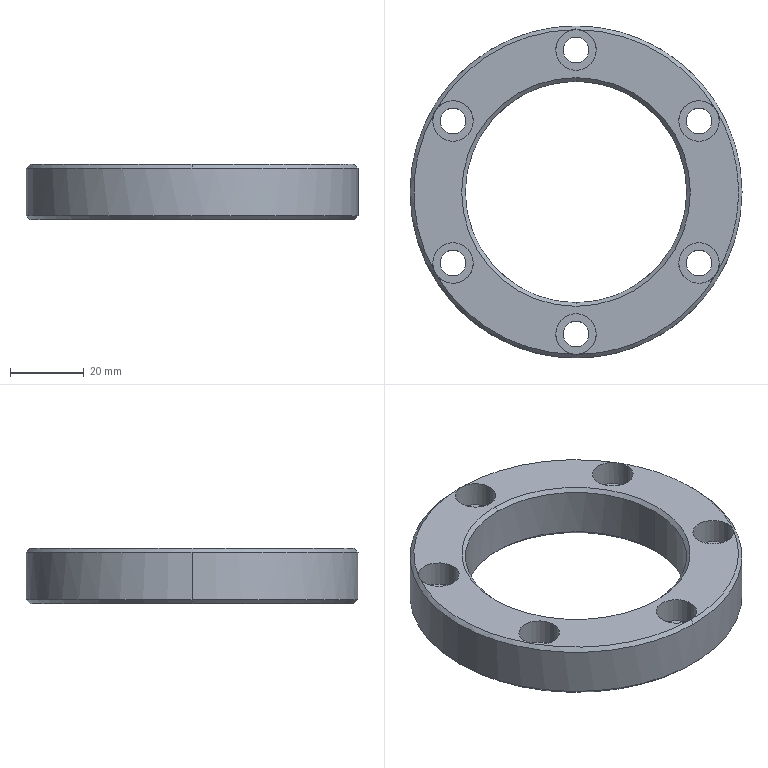Part | STEP file | End Cover | 1 solid | 44 faces | box 90 x 90 x 15 mm | volume 46704 mm3 | cylinder 28 | cone 8 | plane 8 | commonest cylinder face diameters 7 x12 11 x12 60 x2 90 x2
STEP:
#1=CARTESIAN_POINT('',(-29.842,19.25,8.));
#2=VERTEX_POINT('',#1);
#3=CARTESIAN_POINT('',(-36.842,19.25,8.));
#4=VERTEX_POINT('',#3);
#5=CARTESIAN_POINT('',(-33.342,19.25,8.));
#6=DIRECTION('',(0.,0.,-1.));
#7=DIRECTION('',(-1.,0.,0.));
#8=AXIS2_PLACEMENT_3D('',#5,#6,#7);
#9=CIRCLE('',#8,3.5);
#10=EDGE_CURVE('',#2,#4,#9,.T.);
#11=ORIENTED_EDGE('',*,*,#10,.F.);
#12=CARTESIAN_POINT('',(-29.842,19.25,0.));
#13=VERTEX_POINT('',#12);
#14=CARTESIAN_POINT('',(-29.842,19.25,15.));
#15=DIRECTION('',(0.,0.,-1.));
#16=VECTOR('',#15,1000.);
#17=LINE('',#14,#16);
#18=EDGE_CURVE('',#2,#13,#17,.T.);
#19=ORIENTED_EDGE('',*,*,#18,.T.);
#20=CARTESIAN_POINT('',(-36.842,19.25,0.));
#21=VERTEX_POINT('',#20);
#22=CARTESIAN_POINT('',(-33.342,19.25,0.));
#23=DIRECTION('',(0.,0.,-1.));
#24=DIRECTION('',(-1.,0.,0.));
#25=AXIS2_PLACEMENT_3D('',#22,#23,#24);
#26=CIRCLE('',#25,3.5);
#27=EDGE_CURVE('',#13,#21,#26,.T.);
#28=ORIENTED_EDGE('',*,*,#27,.T.);
#29=CARTESIAN_POINT('',(-36.842,19.25,15.));
#30=DIRECTION('',(0.,0.,-1.));
#31=VECTOR('',#30,1000.);
#32=LINE('',#29,#31);
#33=EDGE_CURVE('',#4,#21,#32,.T.);
#34=ORIENTED_EDGE('',*,*,#33,.F.);
#35=EDGE_LOOP('',(#11,#19,#28,#34));
#36=FACE_OUTER_BOUND('',#35,.T.);
#37=CARTESIAN_POINT('',(-33.342,19.25,15.));
#38=DIRECTION('',(0.,0.,-1.));
#39=DIRECTION('',(-1.,0.,0.));
#40=AXIS2_PLACEMENT_3D('',#37,#38,#39);
#41=CYLINDRICAL_SURFACE('',#40,3.5);
#42=ADVANCED_FACE('',(#36),#41,.F.);
#43=CARTESIAN_POINT('',(3.5,-38.5,8.));
#44=VERTEX_POINT('',#43);
#45=CARTESIAN_POINT('',(-3.5,-38.5,8.));
#46=VERTEX_POINT('',#45);
#47=CARTESIAN_POINT('',(0.,-38.5,8.));
#48=DIRECTION('',(0.,0.,-1.));
#49=DIRECTION('',(-1.,0.,0.));
#50=AXIS2_PLACEMENT_3D('',#47,#48,#49);
#51=CIRCLE('',#50,3.5);
#52=EDGE_CURVE('',#44,#46,#51,.T.);
#53=ORIENTED_EDGE('',*,*,#52,.F.);
#54=CARTESIAN_POINT('',(3.5,-38.5,0.));
#55=VERTEX_POINT('',#54);
#56=CARTESIAN_POINT('',(3.5,-38.5,15.));
#57=DIRECTION('',(0.,0.,-1.));
#58=VECTOR('',#57,1000.);
#59=LINE('',#56,#58);
#60=EDGE_CURVE('',#44,#55,#59,.T.);
#61=ORIENTED_EDGE('',*,*,#60,.T.);
#62=CARTESIAN_POINT('',(-3.5,-38.5,0.));
#63=VERTEX_POINT('',#62);
#64=CARTESIAN_POINT('',(0.,-38.5,0.));
#65=DIRECTION('',(0.,0.,-1.));
#66=DIRECTION('',(-1.,0.,0.));
#67=AXIS2_PLACEMENT_3D('',#64,#65,#66);
#68=CIRCLE('',#67,3.5);
#69=EDGE_CURVE('',#55,#63,#68,.T.);
#70=ORIENTED_EDGE('',*,*,#69,.T.);
#71=CARTESIAN_POINT('',(-3.5,-38.5,15.));
#72=DIRECTION('',(0.,0.,-1.));
#73=VECTOR('',#72,1000.);
#74=LINE('',#71,#73);
#75=EDGE_CURVE('',#46,#63,#74,.T.);
#76=ORIENTED_EDGE('',*,*,#75,.F.);
#77=EDGE_LOOP('',(#53,#61,#70,#76));
#78=FACE_OUTER_BOUND('',#77,.T.);
#79=CARTESIAN_POINT('',(0.,-38.5,15.));
#80=DIRECTION('',(0.,0.,-1.));
#81=DIRECTION('',(-1.,0.,0.));
#82=AXIS2_PLACEMENT_3D('',#79,#80,#81);
#83=CYLINDRICAL_SURFACE('',#82,3.5);
#84=ADVANCED_FACE('',(#78),#83,.F.);
#85=CARTESIAN_POINT('',(36.842,19.25,8.));
#86=VERTEX_POINT('',#85);
#87=CARTESIAN_POINT('',(29.842,19.25,8.));
#88=VERTEX_POINT('',#87);
#89=CARTESIAN_POINT('',(33.342,19.25,8.));
#90=DIRECTION('',(0.,0.,-1.));
#91=DIRECTION('',(-1.,0.,0.));
#92=AXIS2_PLACEMENT_3D('',#89,#90,#91);
#93=CIRCLE('',#92,3.5);
#94=EDGE_CURVE('',#86,#88,#93,.T.);
#95=ORIENTED_EDGE('',*,*,#94,.F.);
#96=CARTESIAN_POINT('',(36.842,19.25,0.));
#97=VERTEX_POINT('',#96);
#98=CARTESIAN_POINT('',(36.842,19.25,15.));
#99=DIRECTION('',(0.,0.,-1.));
#100=VECTOR('',#99,1000.);
#101=LINE('',#98,#100);
#102=EDGE_CURVE('',#86,#97,#101,.T.);
#103=ORIENTED_EDGE('',*,*,#102,.T.);
#104=CARTESIAN_POINT('',(29.842,19.25,0.));
#105=VERTEX_POINT('',#104);
#106=CARTESIAN_POINT('',(33.342,19.25,0.));
#107=DIRECTION('',(0.,0.,-1.));
#108=DIRECTION('',(-1.,0.,0.));
#109=AXIS2_PLACEMENT_3D('',#106,#107,#108);
#110=CIRCLE('',#109,3.5);
#111=EDGE_CURVE('',#97,#105,#110,.T.);
#112=ORIENTED_EDGE('',*,*,#111,.T.);
#113=CARTESIAN_POINT('',(29.842,19.25,15.));
#114=DIRECTION('',(0.,0.,-1.));
#115=VECTOR('',#114,1000.);
#116=LINE('',#113,#115);
#117=EDGE_CURVE('',#88,#105,#116,.T.);
#118=ORIENTED_EDGE('',*,*,#117,.F.);
#119=EDGE_LOOP('',(#95,#103,#112,#118));
#120=FACE_OUTER_BOUND('',#119,.T.);
#121=CARTESIAN_POINT('',(33.342,19.25,15.));
#122=DIRECTION('',(0.,0.,-1.));
#123=DIRECTION('',(-1.,0.,0.));
#124=AXIS2_PLACEMENT_3D('',#121,#122,#123);
#125=CYLINDRICAL_SURFACE('',#124,3.5);
#126=ADVANCED_FACE('',(#120),#125,.F.);
#127=CARTESIAN_POINT('',(3.5,38.5,8.));
#128=VERTEX_POINT('',#127);
#129=CARTESIAN_POINT('',(-3.5,38.5,8.));
#130=VERTEX_POINT('',#129);
#131=CARTESIAN_POINT('',(0.,38.5,8.));
#132=DIRECTION('',(0.,0.,-1.));
#133=DIRECTION('',(-1.,0.,0.));
#134=AXIS2_PLACEMENT_3D('',#131,#132,#133);
#135=CIRCLE('',#134,3.5);
#136=EDGE_CURVE('',#128,#130,#135,.T.);
#137=ORIENTED_EDGE('',*,*,#136,.F.);
#138=CARTESIAN_POINT('',(3.5,38.5,0.));
#139=VERTEX_POINT('',#138);
#140=CARTESIAN_POINT('',(3.5,38.5,15.));
#141=DIRECTION('',(0.,0.,-1.));
#142=VECTOR('',#141,1000.);
#143=LINE('',#140,#142);
#144=EDGE_CURVE('',#128,#139,#143,.T.);
#145=ORIENTED_EDGE('',*,*,#144,.T.);
#146=CARTESIAN_POINT('',(-3.5,38.5,0.));
#147=VERTEX_POINT('',#146);
#148=CARTESIAN_POINT('',(0.,38.5,0.));
#149=DIRECTION('',(0.,0.,-1.));
#150=DIRECTION('',(-1.,0.,0.));
#151=AXIS2_PLACEMENT_3D('',#148,#149,#150);
#152=CIRCLE('',#151,3.5);
#153=EDGE_CURVE('',#139,#147,#152,.T.);
#154=ORIENTED_EDGE('',*,*,#153,.T.);
#155=CARTESIAN_POINT('',(-3.5,38.5,15.));
#156=DIRECTION('',(0.,0.,-1.));
#157=VECTOR('',#156,1000.);
#158=LINE('',#155,#157);
#159=EDGE_CURVE('',#130,#147,#158,.T.);
#160=ORIENTED_EDGE('',*,*,#159,.F.);
#161=EDGE_LOOP('',(#137,#145,#154,#160));
#162=FACE_OUTER_BOUND('',#161,.T.);
#163=CARTESIAN_POINT('',(0.,38.5,15.));
#164=DIRECTION('',(0.,0.,-1.));
#165=DIRECTION('',(-1.,0.,0.));
#166=AXIS2_PLACEMENT_3D('',#163,#164,#165);
#167=CYLINDRICAL_SURFACE('',#166,3.5);
#168=ADVANCED_FACE('',(#162),#167,.F.);
#169=CARTESIAN_POINT('',(36.842,-19.25,8.));
#170=VERTEX_POINT('',#169);
#171=CARTESIAN_POINT('',(29.842,-19.25,8.));
#172=VERTEX_POINT('',#171);
#173=CARTESIAN_POINT('',(33.342,-19.25,8.));
#174=DIRECTION('',(0.,0.,-1.));
#175=DIRECTION('',(-1.,0.,0.));
#176=AXIS2_PLACEMENT_3D('',#173,#174,#175);
#177=CIRCLE('',#176,3.5);
#178=EDGE_CURVE('',#170,#172,#177,.T.);
#179=ORIENTED_EDGE('',*,*,#178,.F.);
#180=CARTESIAN_POINT('',(36.842,-19.25,0.));
#181=VERTEX_POINT('',#180);
#182=CARTESIAN_POINT('',(36.842,-19.25,15.));
#183=DIRECTION('',(0.,0.,-1.));
#184=VECTOR('',#183,1000.);
#185=LINE('',#182,#184);
#186=EDGE_CURVE('',#170,#181,#185,.T.);
#187=ORIENTED_EDGE('',*,*,#186,.T.);
#188=CARTESIAN_POINT('',(29.842,-19.25,0.));
#189=VERTEX_POINT('',#188);
#190=CARTESIAN_POINT('',(33.342,-19.25,0.));
#191=DIRECTION('',(0.,0.,-1.));
#192=DIRECTION('',(-1.,0.,0.));
#193=AXIS2_PLACEMENT_3D('',#190,#191,#192);
#194=CIRCLE('',#193,3.5);
#195=EDGE_CURVE('',#181,#189,#194,.T.);
#196=ORIENTED_EDGE('',*,*,#195,.T.);
#197=CARTESIAN_POINT('',(29.842,-19.25,15.));
#198=DIRECTION('',(0.,0.,-1.));
#199=VECTOR('',#198,1000.);
#200=LINE('',#197,#199);
#201=EDGE_CURVE('',#172,#189,#200,.T.);
#202=ORIENTED_EDGE('',*,*,#201,.F.);
#203=EDGE_LOOP('',(#179,#187,#196,#202));
#204=FACE_OUTER_BOUND('',#203,.T.);
#205=CARTESIAN_POINT('',(33.342,-19.25,15.));
#206=DIRECTION('',(0.,0.,-1.));
#207=DIRECTION('',(-1.,0.,0.));
#208=AXIS2_PLACEMENT_3D('',#205,#206,#207);
#209=CYLINDRICAL_SURFACE('',#208,3.5);
#210=ADVANCED_FACE('',(#204),#209,.F.);
#211=CARTESIAN_POINT('',(-29.842,-19.25,8.));
#212=VERTEX_POINT('',#211);
#213=CARTESIAN_POINT('',(-36.842,-19.25,8.));
#214=VERTEX_POINT('',#213);
#215=CARTESIAN_POINT('',(-33.342,-19.25,8.));
#216=DIRECTION('',(0.,0.,-1.));
#217=DIRECTION('',(-1.,0.,0.));
#218=AXIS2_PLACEMENT_3D('',#215,#216,#217);
#219=CIRCLE('',#218,3.5);
#220=EDGE_CURVE('',#212,#214,#219,.T.);
#221=ORIENTED_EDGE('',*,*,#220,.F.);
#222=CARTESIAN_POINT('',(-29.842,-19.25,0.));
#223=VERTEX_POINT('',#222);
#224=CARTESIAN_POINT('',(-29.842,-19.25,15.));
#225=DIRECTION('',(0.,0.,-1.));
#226=VECTOR('',#225,1000.);
#227=LINE('',#224,#226);
#228=EDGE_CURVE('',#212,#223,#227,.T.);
#229=ORIENTED_EDGE('',*,*,#228,.T.);
#230=CARTESIAN_POINT('',(-36.842,-19.25,0.));
#231=VERTEX_POINT('',#230);
#232=CARTESIAN_POINT('',(-33.342,-19.25,0.));
#233=DIRECTION('',(0.,0.,-1.));
#234=DIRECTION('',(-1.,0.,0.));
#235=AXIS2_PLACEMENT_3D('',#232,#233,#234);
#236=CIRCLE('',#235,3.5);
#237=EDGE_CURVE('',#223,#231,#236,.T.);
#238=ORIENTED_EDGE('',*,*,#237,.T.);
#239=CARTESIAN_POINT('',(-36.842,-19.25,15.));
#240=DIRECTION('',(0.,0.,-1.));
#241=VECTOR('',#240,1000.);
#242=LINE('',#239,#241);
#243=EDGE_CURVE('',#214,#231,#242,.T.);
#244=ORIENTED_EDGE('',*,*,#243,.F.);
#245=EDGE_LOOP('',(#221,#229,#238,#244));
#246=FACE_OUTER_BOUND('',#245,.T.);
#247=CARTESIAN_POINT('',(-33.342,-19.25,15.));
#248=DIRECTION('',(0.,0.,-1.));
#249=DIRECTION('',(-1.,0.,0.));
#250=AXIS2_PLACEMENT_3D('',#247,#248,#249);
#251=CYLINDRICAL_SURFACE('',#250,3.5);
#252=ADVANCED_FACE('',(#246),#251,.F.);
#253=CARTESIAN_POINT('',(30.,0.,1.));
#254=VERTEX_POINT('',#253);
#255=CARTESIAN_POINT('',(-30.,0.,1.));
#256=VERTEX_POINT('',#255);
#257=CARTESIAN_POINT('',(0.,0.,1.));
#258=DIRECTION('',(0.,0.,-1.));
#259=DIRECTION('',(-1.,0.,0.));
#260=AXIS2_PLACEMENT_3D('',#257,#258,#259);
#261=CIRCLE('',#260,30.);
#262=EDGE_CURVE('',#254,#256,#261,.T.);
#263=ORIENTED_EDGE('',*,*,#262,.F.);
#264=CARTESIAN_POINT('',(31.,0.,0.));
#265=VERTEX_POINT('',#264);
#266=CARTESIAN_POINT('',(31.,0.,0.));
#267=DIRECTION('',(0.7071,0.,-0.7071));
#268=VECTOR('',#267,1000.);
#269=LINE('',#266,#268);
#270=EDGE_CURVE('',#254,#265,#269,.T.);
#271=ORIENTED_EDGE('',*,*,#270,.T.);
#272=CARTESIAN_POINT('',(-31.,0.,0.));
#273=VERTEX_POINT('',#272);
#274=CARTESIAN_POINT('',(0.,0.,0.));
#275=DIRECTION('',(0.,0.,-1.));
#276=DIRECTION('',(-1.,0.,0.));
#277=AXIS2_PLACEMENT_3D('',#274,#275,#276);
#278=CIRCLE('',#277,31.);
#279=EDGE_CURVE('',#265,#273,#278,.T.);
#280=ORIENTED_EDGE('',*,*,#279,.T.);
#281=CARTESIAN_POINT('',(-31.,0.,0.));
#282=DIRECTION('',(-0.7071,0.,-0.7071));
#283=VECTOR('',#282,1000.);
#284=LINE('',#281,#283);
#285=EDGE_CURVE('',#256,#273,#284,.T.);
#286=ORIENTED_EDGE('',*,*,#285,.F.);
#287=EDGE_LOOP('',(#263,#271,#280,#286));
#288=FACE_OUTER_BOUND('',#287,.T.);
#289=CARTESIAN_POINT('',(0.,0.,0.));
#290=DIRECTION('',(0.,0.,-1.));
#291=DIRECTION('',(-1.,0.,0.));
#292=AXIS2_PLACEMENT_3D('',#289,#290,#291);
#293=CONICAL_SURFACE('',#292,31.,0.7854);
#294=ADVANCED_FACE('',(#288),#293,.F.);
#295=CARTESIAN_POINT('',(44.,0.,0.));
#296=VERTEX_POINT('',#295);
#297=CARTESIAN_POINT('',(-44.,0.,0.));
#298=VERTEX_POINT('',#297);
#299=CARTESIAN_POINT('',(0.,0.,0.));
#300=DIRECTION('',(0.,0.,1.));
#301=DIRECTION('',(1.,0.,0.));
#302=AXIS2_PLACEMENT_3D('',#299,#300,#301);
#303=CIRCLE('',#302,44.);
#304=EDGE_CURVE('',#296,#298,#303,.T.);
#305=ORIENTED_EDGE('',*,*,#304,.T.);
#306=CARTESIAN_POINT('',(-45.,0.,1.));
#307=VERTEX_POINT('',#306);
#308=CARTESIAN_POINT('',(-45.,0.,1.));
#309=DIRECTION('',(-0.7071,0.,0.7071));
#310=VECTOR('',#309,1000.);
#311=LINE('',#308,#310);
#312=EDGE_CURVE('',#298,#307,#311,.T.);
#313=ORIENTED_EDGE('',*,*,#312,.T.);
#314=CARTESIAN_POINT('',(45.,0.,1.));
#315=VERTEX_POINT('',#314);
#316=CARTESIAN_POINT('',(0.,0.,1.));
#317=DIRECTION('',(0.,0.,-1.));
#318=DIRECTION('',(1.,0.,0.));
#319=AXIS2_PLACEMENT_3D('',#316,#317,#318);
#320=CIRCLE('',#319,45.);
#321=EDGE_CURVE('',#307,#315,#320,.T.);
#322=ORIENTED_EDGE('',*,*,#321,.T.);
#323=CARTESIAN_POINT('',(45.,0.,1.));
#324=DIRECTION('',(0.7071,0.,0.7071));
#325=VECTOR('',#324,1000.);
#326=LINE('',#323,#325);
#327=EDGE_CURVE('',#296,#315,#326,.T.);
#328=ORIENTED_EDGE('',*,*,#327,.F.);
#329=EDGE_LOOP('',(#305,#313,#322,#328));
#330=FACE_OUTER_BOUND('',#329,.T.);
#331=CARTESIAN_POINT('',(0.,0.,1.));
#332=DIRECTION('',(0.,0.,1.));
#333=DIRECTION('',(1.,0.,0.));
#334=AXIS2_PLACEMENT_3D('',#331,#332,#333);
#335=CONICAL_SURFACE('',#334,45.,0.7854);
#336=ADVANCED_FACE('',(#330),#335,.T.);
#337=CARTESIAN_POINT('',(30.,0.,14.));
#338=VERTEX_POINT('',#337);
#339=CARTESIAN_POINT('',(0.,-30.,14.));
#340=VERTEX_POINT('',#339);
#341=CARTESIAN_POINT('',(0.,0.,14.));
#342=DIRECTION('',(0.,0.,-1.));
#343=DIRECTION('',(-1.,0.,0.));
#344=AXIS2_PLACEMENT_3D('',#341,#342,#343);
#345=CIRCLE('',#344,30.);
#346=EDGE_CURVE('',#338,#340,#345,.T.);
#347=ORIENTED_EDGE('',*,*,#346,.F.);
#348=CARTESIAN_POINT('',(30.,0.,15.));
#349=DIRECTION('',(0.,0.,-1.));
#350=VECTOR('',#349,1000.);
#351=LINE('',#348,#350);
#352=EDGE_CURVE('',#338,#254,#351,.T.);
#353=ORIENTED_EDGE('',*,*,#352,.T.);
#354=ORIENTED_EDGE('',*,*,#262,.T.);
#355=CARTESIAN_POINT('',(-30.,0.,14.));
#356=VERTEX_POINT('',#355);
#357=CARTESIAN_POINT('',(-30.,0.,15.));
#358=DIRECTION('',(0.,0.,-1.));
#359=VECTOR('',#358,1000.);
#360=LINE('',#357,#359);
#361=EDGE_CURVE('',#356,#256,#360,.T.);
#362=ORIENTED_EDGE('',*,*,#361,.F.);
#363=CARTESIAN_POINT('',(0.,0.,14.));
#364=DIRECTION('',(0.,0.,-1.));
#365=DIRECTION('',(-1.,0.,0.));
#366=AXIS2_PLACEMENT_3D('',#363,#364,#365);
#367=CIRCLE('',#366,30.);
#368=EDGE_CURVE('',#340,#356,#367,.T.);
#369=ORIENTED_EDGE('',*,*,#368,.F.);
#370=EDGE_LOOP('',(#347,#353,#354,#362,#369));
#371=FACE_OUTER_BOUND('',#370,.T.);
#372=CARTESIAN_POINT('',(0.,0.,15.));
#373=DIRECTION('',(0.,0.,-1.));
#374=DIRECTION('',(-1.,0.,0.));
#375=AXIS2_PLACEMENT_3D('',#372,#373,#374);
#376=CYLINDRICAL_SURFACE('',#375,30.);
#377=ADVANCED_FACE('',(#371),#376,.F.);
#378=CARTESIAN_POINT('',(0.,45.,14.));
#379=VERTEX_POINT('',#378);
#380=CARTESIAN_POINT('',(45.,0.,14.));
#381=VERTEX_POINT('',#380);
#382=CARTESIAN_POINT('',(0.,0.,14.));
#383=DIRECTION('',(0.,0.,-1.));
#384=DIRECTION('',(-1.,0.,0.));
#385=AXIS2_PLACEMENT_3D('',#382,#383,#384);
#386=CIRCLE('',#385,45.);
#387=EDGE_CURVE('',#379,#381,#386,.T.);
#388=ORIENTED_EDGE('',*,*,#387,.T.);
#389=CARTESIAN_POINT('',(45.,0.,15.));
#390=DIRECTION('',(0.,0.,-1.));
#391=VECTOR('',#390,1000.);
#392=LINE('',#389,#391);
#393=EDGE_CURVE('',#381,#315,#392,.T.);
#394=ORIENTED_EDGE('',*,*,#393,.T.);
#395=ORIENTED_EDGE('',*,*,#321,.F.);
#396=CARTESIAN_POINT('',(-45.,0.,14.));
#397=VERTEX_POINT('',#396);
#398=CARTESIAN_POINT('',(-45.,0.,15.));
#399=DIRECTION('',(0.,0.,-1.));
#400=VECTOR('',#399,1000.);
#401=LINE('',#398,#400);
#402=EDGE_CURVE('',#397,#307,#401,.T.);
#403=ORIENTED_EDGE('',*,*,#402,.F.);
#404=CARTESIAN_POINT('',(0.,0.,14.));
#405=DIRECTION('',(0.,0.,-1.));
#406=DIRECTION('',(-1.,0.,0.));
#407=AXIS2_PLACEMENT_3D('',#404,#405,#406);
#408=CIRCLE('',#407,45.);
#409=EDGE_CURVE('',#397,#379,#408,.T.);
#410=ORIENTED_EDGE('',*,*,#409,.T.);
#411=EDGE_LOOP('',(#388,#394,#395,#403,#410));
#412=FACE_OUTER_BOUND('',#411,.T.);
#413=CARTESIAN_POINT('',(0.,0.,15.));
#414=DIRECTION('',(0.,0.,-1.));
#415=DIRECTION('',(-1.,0.,0.));
#416=AXIS2_PLACEMENT_3D('',#413,#414,#415);
#417=CYLINDRICAL_SURFACE('',#416,45.);
#418=ADVANCED_FACE('',(#412),#417,.T.);
#419=CARTESIAN_POINT('',(-38.842,19.25,8.));
#420=VERTEX_POINT('',#419);
#421=CARTESIAN_POINT('',(-27.842,19.25,8.));
#422=VERTEX_POINT('',#421);
#423=CARTESIAN_POINT('',(-33.342,19.25,8.));
#424=DIRECTION('',(0.,0.,1.));
#425=DIRECTION('',(1.,0.,0.));
#426=AXIS2_PLACEMENT_3D('',#423,#424,#425);
#427=CIRCLE('',#426,5.5);
#428=EDGE_CURVE('',#420,#422,#427,.T.);
#429=ORIENTED_EDGE('',*,*,#428,.F.);
#430=CARTESIAN_POINT('',(-38.842,19.25,15.));
#431=VERTEX_POINT('',#430);
#432=CARTESIAN_POINT('',(-38.842,19.25,8.));
#433=DIRECTION('',(0.,0.,1.));
#434=VECTOR('',#433,1000.);
#435=LINE('',#432,#434);
#436=EDGE_CURVE('',#420,#431,#435,.T.);
#437=ORIENTED_EDGE('',*,*,#436,.T.);
#438=CARTESIAN_POINT('',(-27.842,19.25,15.));
#439=VERTEX_POINT('',#438);
#440=CARTESIAN_POINT('',(-33.342,19.25,15.));
#441=DIRECTION('',(0.,0.,-1.));
#442=DIRECTION('',(1.,0.,0.));
#443=AXIS2_PLACEMENT_3D('',#440,#441,#442);
#444=CIRCLE('',#443,5.5);
#445=EDGE_CURVE('',#439,#431,#444,.T.);
#446=ORIENTED_EDGE('',*,*,#445,.F.);
#447=CARTESIAN_POINT('',(-27.842,19.25,8.));
#448=DIRECTION('',(0.,0.,1.));
#449=VECTOR('',#448,1000.);
#450=LINE('',#447,#449);
#451=EDGE_CURVE('',#422,#439,#450,.T.);
#452=ORIENTED_EDGE('',*,*,#451,.F.);
#453=EDGE_LOOP('',(#429,#437,#446,#452));
#454=FACE_OUTER_BOUND('',#453,.T.);
#455=CARTESIAN_POINT('',(-33.342,19.25,8.));
#456=DIRECTION('',(0.,0.,1.));
#457=DIRECTION('',(1.,0.,0.));
#458=AXIS2_PLACEMENT_3D('',#455,#456,#457);
#459=CYLINDRICAL_SURFACE('',#458,5.5);
#460=ADVANCED_FACE('',(#454),#459,.F.);
#461=CARTESIAN_POINT('',(-5.5,-38.5,8.));
#462=VERTEX_POINT('',#461);
#463=CARTESIAN_POINT('',(5.5,-38.5,8.));
#464=VERTEX_POINT('',#463);
#465=CARTESIAN_POINT('',(0.,-38.5,8.));
#466=DIRECTION('',(0.,0.,1.));
#467=DIRECTION('',(1.,0.,0.));
#468=AXIS2_PLACEMENT_3D('',#465,#466,#467);
#469=CIRCLE('',#468,5.5);
#470=EDGE_CURVE('',#462,#464,#469,.T.);
#471=ORIENTED_EDGE('',*,*,#470,.F.);
#472=CARTESIAN_POINT('',(-5.5,-38.5,15.));
#473=VERTEX_POINT('',#472);
#474=CARTESIAN_POINT('',(-5.5,-38.5,8.));
#475=DIRECTION('',(0.,0.,1.));
#476=VECTOR('',#475,1000.);
#477=LINE('',#474,#476);
#478=EDGE_CURVE('',#462,#473,#477,.T.);
#479=ORIENTED_EDGE('',*,*,#478,.T.);
#480=CARTESIAN_POINT('',(0.,-44.,15.));
#481=VERTEX_POINT('',#480);
#482=CARTESIAN_POINT('',(0.,-38.5,15.));
#483=DIRECTION('',(0.,0.,-1.));
#484=DIRECTION('',(1.,0.,0.));
#485=AXIS2_PLACEMENT_3D('',#482,#483,#484);
#486=CIRCLE('',#485,5.5);
#487=EDGE_CURVE('',#481,#473,#486,.T.);
#488=ORIENTED_EDGE('',*,*,#487,.F.);
#489=CARTESIAN_POINT('',(5.5,-38.5,15.));
#490=VERTEX_POINT('',#489);
#491=CARTESIAN_POINT('',(0.,-38.5,15.));
#492=DIRECTION('',(0.,0.,-1.));
#493=DIRECTION('',(1.,0.,0.));
#494=AXIS2_PLACEMENT_3D('',#491,#492,#493);
#495=CIRCLE('',#494,5.5);
#496=EDGE_CURVE('',#490,#481,#495,.T.);
#497=ORIENTED_EDGE('',*,*,#496,.F.);
#498=CARTESIAN_POINT('',(5.5,-38.5,8.));
#499=DIRECTION('',(0.,0.,1.));
#500=VECTOR('',#499,1000.);
#501=LINE('',#498,#500);
#502=EDGE_CURVE('',#464,#490,#501,.T.);
#503=ORIENTED_EDGE('',*,*,#502,.F.);
#504=EDGE_LOOP('',(#471,#479,#488,#497,#503));
#505=FACE_OUTER_BOUND('',#504,.T.);
#506=CARTESIAN_POINT('',(0.,-38.5,8.));
#507=DIRECTION('',(0.,0.,1.));
#508=DIRECTION('',(1.,0.,0.));
#509=AXIS2_PLACEMENT_3D('',#506,#507,#508);
#510=CYLINDRICAL_SURFACE('',#509,5.5);
#511=ADVANCED_FACE('',(#505),#510,.F.);
#512=CARTESIAN_POINT('',(27.842,19.25,8.));
#513=VERTEX_POINT('',#512);
#514=CARTESIAN_POINT('',(38.842,19.25,8.));
#515=VERTEX_POINT('',#514);
#516=CARTESIAN_POINT('',(33.342,19.25,8.));
#517=DIRECTION('',(0.,0.,1.));
#518=DIRECTION('',(1.,0.,0.));
#519=AXIS2_PLACEMENT_3D('',#516,#517,#518);
#520=CIRCLE('',#519,5.5);
#521=EDGE_CURVE('',#513,#515,#520,.T.);
#522=ORIENTED_EDGE('',*,*,#521,.F.);
#523=CARTESIAN_POINT('',(27.842,19.25,15.));
#524=VERTEX_POINT('',#523);
#525=CARTESIAN_POINT('',(27.842,19.25,8.));
#526=DIRECTION('',(0.,0.,1.));
#527=VECTOR('',#526,1000.);
#528=LINE('',#525,#527);
#529=EDGE_CURVE('',#513,#524,#528,.T.);
#530=ORIENTED_EDGE('',*,*,#529,.T.);
#531=CARTESIAN_POINT('',(38.842,19.25,15.));
#532=VERTEX_POINT('',#531);
#533=CARTESIAN_POINT('',(33.342,19.25,15.));
#534=DIRECTION('',(0.,0.,-1.));
#535=DIRECTION('',(1.,0.,0.));
#536=AXIS2_PLACEMENT_3D('',#533,#534,#535);
#537=CIRCLE('',#536,5.5);
#538=EDGE_CURVE('',#532,#524,#537,.T.);
#539=ORIENTED_EDGE('',*,*,#538,.F.);
#540=CARTESIAN_POINT('',(38.842,19.25,8.));
#541=DIRECTION('',(0.,0.,1.));
#542=VECTOR('',#541,1000.);
#543=LINE('',#540,#542);
#544=EDGE_CURVE('',#515,#532,#543,.T.);
#545=ORIENTED_EDGE('',*,*,#544,.F.);
#546=EDGE_LOOP('',(#522,#530,#539,#545));
#547=FACE_OUTER_BOUND('',#546,.T.);
#548=CARTESIAN_POINT('',(33.342,19.25,8.));
#549=DIRECTION('',(0.,0.,1.));
#550=DIRECTION('',(1.,0.,0.));
#551=AXIS2_PLACEMENT_3D('',#548,#549,#550);
#552=CYLINDRICAL_SURFACE('',#551,5.5);
#553=ADVANCED_FACE('',(#547),#552,.F.);
#554=CARTESIAN_POINT('',(-5.5,38.5,8.));
#555=VERTEX_POINT('',#554);
#556=CARTESIAN_POINT('',(5.5,38.5,8.));
#557=VERTEX_POINT('',#556);
#558=CARTESIAN_POINT('',(0.,38.5,8.));
#559=DIRECTION('',(0.,0.,1.));
#560=DIRECTION('',(1.,0.,0.));
#561=AXIS2_PLACEMENT_3D('',#558,#559,#560);
#562=CIRCLE('',#561,5.5);
#563=EDGE_CURVE('',#555,#557,#562,.T.);
#564=ORIENTED_EDGE('',*,*,#563,.F.);
#565=CARTESIAN_POINT('',(-5.5,38.5,15.));
#566=VERTEX_POINT('',#565);
#567=CARTESIAN_POINT('',(-5.5,38.5,8.));
#568=DIRECTION('',(0.,0.,1.));
#569=VECTOR('',#568,1000.);
#570=LINE('',#567,#569);
#571=EDGE_CURVE('',#555,#566,#570,.T.);
#572=ORIENTED_EDGE('',*,*,#571,.T.);
#573=CARTESIAN_POINT('',(5.5,38.5,15.));
#574=VERTEX_POINT('',#573);
#575=CARTESIAN_POINT('',(0.,38.5,15.));
#576=DIRECTION('',(0.,0.,-1.));
#577=DIRECTION('',(1.,0.,0.));
#578=AXIS2_PLACEMENT_3D('',#575,#576,#577);
#579=CIRCLE('',#578,5.5);
#580=EDGE_CURVE('',#574,#566,#579,.T.);
#581=ORIENTED_EDGE('',*,*,#580,.F.);
#582=CARTESIAN_POINT('',(5.5,38.5,8.));
#583=DIRECTION('',(0.,0.,1.));
#584=VECTOR('',#583,1000.);
#585=LINE('',#582,#584);
#586=EDGE_CURVE('',#557,#574,#585,.T.);
#587=ORIENTED_EDGE('',*,*,#586,.F.);
#588=EDGE_LOOP('',(#564,#572,#581,#587));
#589=FACE_OUTER_BOUND('',#588,.T.);
#590=CARTESIAN_POINT('',(0.,38.5,8.));
#591=DIRECTION('',(0.,0.,1.));
#592=DIRECTION('',(1.,0.,0.));
#593=AXIS2_PLACEMENT_3D('',#590,#591,#592);
#594=CYLINDRICAL_SURFACE('',#593,5.5);
#595=ADVANCED_FACE('',(#589),#594,.F.);
#596=CARTESIAN_POINT('',(27.842,-19.25,8.));
#597=VERTEX_POINT('',#596);
#598=CARTESIAN_POINT('',(38.842,-19.25,8.));
#599=VERTEX_POINT('',#598);
#600=CARTESIAN_POINT('',(33.342,-19.25,8.));
#601=DIRECTION('',(0.,0.,1.));
#602=DIRECTION('',(1.,0.,0.));
#603=AXIS2_PLACEMENT_3D('',#600,#601,#602);
#604=CIRCLE('',#603,5.5);
#605=EDGE_CURVE('',#597,#599,#604,.T.);
#606=ORIENTED_EDGE('',*,*,#605,.F.);
#607=CARTESIAN_POINT('',(27.842,-19.25,15.));
#608=VERTEX_POINT('',#607);
#609=CARTESIAN_POINT('',(27.842,-19.25,8.));
#610=DIRECTION('',(0.,0.,1.));
#611=VECTOR('',#610,1000.);
#612=LINE('',#609,#611);
#613=EDGE_CURVE('',#597,#608,#612,.T.);
#614=ORIENTED_EDGE('',*,*,#613,.T.);
#615=CARTESIAN_POINT('',(38.105,-22.,15.));
#616=VERTEX_POINT('',#615);
#617=CARTESIAN_POINT('',(33.342,-19.25,15.));
#618=DIRECTION('',(0.,0.,-1.));
#619=DIRECTION('',(1.,0.,0.));
#620=AXIS2_PLACEMENT_3D('',#617,#618,#619);
#621=CIRCLE('',#620,5.5);
#622=EDGE_CURVE('',#616,#608,#621,.T.);
#623=ORIENTED_EDGE('',*,*,#622,.F.);
#624=CARTESIAN_POINT('',(38.842,-19.25,15.));
#625=VERTEX_POINT('',#624);
#626=CARTESIAN_POINT('',(33.342,-19.25,15.));
#627=DIRECTION('',(0.,0.,-1.));
#628=DIRECTION('',(1.,0.,0.));
#629=AXIS2_PLACEMENT_3D('',#626,#627,#628);
#630=CIRCLE('',#629,5.5);
#631=EDGE_CURVE('',#625,#616,#630,.T.);
#632=ORIENTED_EDGE('',*,*,#631,.F.);
#633=CARTESIAN_POINT('',(38.842,-19.25,8.));
#634=DIRECTION('',(0.,0.,1.));
#635=VECTOR('',#634,1000.);
#636=LINE('',#633,#635);
#637=EDGE_CURVE('',#599,#625,#636,.T.);
#638=ORIENTED_EDGE('',*,*,#637,.F.);
#639=EDGE_LOOP('',(#606,#614,#623,#632,#638));
#640=FACE_OUTER_BOUND('',#639,.T.);
#641=CARTESIAN_POINT('',(33.342,-19.25,8.));
#642=DIRECTION('',(0.,0.,1.));
#643=DIRECTION('',(1.,0.,0.));
#644=AXIS2_PLACEMENT_3D('',#641,#642,#643);
#645=CYLINDRICAL_SURFACE('',#644,5.5);
#646=ADVANCED_FACE('',(#640),#645,.F.);
#647=CARTESIAN_POINT('',(-38.842,-19.25,8.));
#648=VERTEX_POINT('',#647);
#649=CARTESIAN_POINT('',(-27.842,-19.25,8.));
#650=VERTEX_POINT('',#649);
#651=CARTESIAN_POINT('',(-33.342,-19.25,8.));
#652=DIRECTION('',(0.,0.,1.));
#653=DIRECTION('',(1.,0.,0.));
#654=AXIS2_PLACEMENT_3D('',#651,#652,#653);
#655=CIRCLE('',#654,5.5);
#656=EDGE_CURVE('',#648,#650,#655,.T.);
#657=ORIENTED_EDGE('',*,*,#656,.F.);
#658=CARTESIAN_POINT('',(-38.842,-19.25,15.));
#659=VERTEX_POINT('',#658);
#660=CARTESIAN_POINT('',(-38.842,-19.25,8.));
#661=DIRECTION('',(0.,0.,1.));
#662=VECTOR('',#661,1000.);
#663=LINE('',#660,#662);
#664=EDGE_CURVE('',#648,#659,#663,.T.);
#665=ORIENTED_EDGE('',*,*,#664,.T.);
#666=CARTESIAN_POINT('',(-38.105,-22.,15.));
#667=VERTEX_POINT('',#666);
#668=CARTESIAN_POINT('',(-33.342,-19.25,15.));
#669=DIRECTION('',(0.,0.,-1.));
#670=DIRECTION('',(1.,0.,0.));
#671=AXIS2_PLACEMENT_3D('',#668,#669,#670);
#672=CIRCLE('',#671,5.5);
#673=EDGE_CURVE('',#667,#659,#672,.T.);
#674=ORIENTED_EDGE('',*,*,#673,.F.);
#675=CARTESIAN_POINT('',(-27.842,-19.25,15.));
#676=VERTEX_POINT('',#675);
#677=CARTESIAN_POINT('',(-33.342,-19.25,15.));
#678=DIRECTION('',(0.,0.,-1.));
#679=DIRECTION('',(1.,0.,0.));
#680=AXIS2_PLACEMENT_3D('',#677,#678,#679);
#681=CIRCLE('',#680,5.5);
#682=EDGE_CURVE('',#676,#667,#681,.T.);
#683=ORIENTED_EDGE('',*,*,#682,.F.);
#684=CARTESIAN_POINT('',(-27.842,-19.25,8.));
#685=DIRECTION('',(0.,0.,1.));
#686=VECTOR('',#685,1000.);
#687=LINE('',#684,#686);
#688=EDGE_CURVE('',#650,#676,#687,.T.);
#689=ORIENTED_EDGE('',*,*,#688,.F.);
#690=EDGE_LOOP('',(#657,#665,#674,#683,#689));
#691=FACE_OUTER_BOUND('',#690,.T.);
#692=CARTESIAN_POINT('',(-33.342,-19.25,8.));
#693=DIRECTION('',(0.,0.,1.));
#694=DIRECTION('',(1.,0.,0.));
#695=AXIS2_PLACEMENT_3D('',#692,#693,#694);
#696=CYLINDRICAL_SURFACE('',#695,5.5);
#697=ADVANCED_FACE('',(#691),#696,.F.);
#698=ORIENTED_EDGE('',*,*,#368,.T.);
#699=CARTESIAN_POINT('',(0.,30.,14.));
#700=VERTEX_POINT('',#699);
#701=CARTESIAN_POINT('',(0.,0.,14.));
#702=DIRECTION('',(0.,0.,-1.));
#703=DIRECTION('',(-1.,0.,0.));
#704=AXIS2_PLACEMENT_3D('',#701,#702,#703);
#705=CIRCLE('',#704,30.);
#706=EDGE_CURVE('',#356,#700,#705,.T.);
#707=ORIENTED_EDGE('',*,*,#706,.T.);
#708=CARTESIAN_POINT('',(0.,31.,15.));
#709=VERTEX_POINT('',#708);
#710=CARTESIAN_POINT('',(0.,31.,15.));
#711=DIRECTION('',(0.,0.7071,0.7071));
#712=VECTOR('',#711,1000.);
#713=LINE('',#710,#712);
#714=EDGE_CURVE('',#700,#709,#713,.T.);
#715=ORIENTED_EDGE('',*,*,#714,.T.);
#716=CARTESIAN_POINT('',(0.,-31.,15.));
#717=VERTEX_POINT('',#716);
#718=CARTESIAN_POINT('',(0.,0.,15.));
#719=DIRECTION('',(0.,0.,-1.));
#720=DIRECTION('',(0.,-1.,0.));
#721=AXIS2_PLACEMENT_3D('',#718,#719,#720);
#722=CIRCLE('',#721,31.);
#723=EDGE_CURVE('',#717,#709,#722,.T.);
#724=ORIENTED_EDGE('',*,*,#723,.F.);
#725=CARTESIAN_POINT('',(0.,-31.,15.));
#726=DIRECTION('',(0.,-0.7071,0.7071));
#727=VECTOR('',#726,1000.);
#728=LINE('',#725,#727);
#729=EDGE_CURVE('',#340,#717,#728,.T.);
#730=ORIENTED_EDGE('',*,*,#729,.F.);
#731=EDGE_LOOP('',(#698,#707,#715,#724,#730));
#732=FACE_OUTER_BOUND('',#731,.T.);
#733=CARTESIAN_POINT('',(0.,0.,15.));
#734=DIRECTION('',(0.,0.,1.));
#735=DIRECTION('',(0.,-1.,0.));
#736=AXIS2_PLACEMENT_3D('',#733,#734,#735);
#737=CONICAL_SURFACE('',#736,31.,0.7854);
#738=ADVANCED_FACE('',(#732),#737,.F.);
#739=CARTESIAN_POINT('',(0.,0.,15.));
#740=DIRECTION('',(0.,0.,-1.));
#741=DIRECTION('',(0.,1.,0.));
#742=AXIS2_PLACEMENT_3D('',#739,#740,#741);
#743=CIRCLE('',#742,44.);
#744=EDGE_CURVE('',#616,#481,#743,.T.);
#745=ORIENTED_EDGE('',*,*,#744,.T.);
#746=CARTESIAN_POINT('',(0.,-45.,14.));
#747=VERTEX_POINT('',#746);
#748=CARTESIAN_POINT('',(0.,-45.,14.));
#749=DIRECTION('',(0.,-0.7071,-0.7071));
#750=VECTOR('',#749,1000.);
#751=LINE('',#748,#750);
#752=EDGE_CURVE('',#481,#747,#751,.T.);
#753=ORIENTED_EDGE('',*,*,#752,.T.);
#754=CARTESIAN_POINT('',(0.,0.,14.));
#755=DIRECTION('',(0.,0.,-1.));
#756=DIRECTION('',(-1.,0.,0.));
#757=AXIS2_PLACEMENT_3D('',#754,#755,#756);
#758=CIRCLE('',#757,45.);
#759=EDGE_CURVE('',#381,#747,#758,.T.);
#760=ORIENTED_EDGE('',*,*,#759,.F.);
#761=ORIENTED_EDGE('',*,*,#387,.F.);
#762=CARTESIAN_POINT('',(0.,44.,15.));
#763=VERTEX_POINT('',#762);
#764=CARTESIAN_POINT('',(0.,45.,14.));
#765=DIRECTION('',(0.,0.7071,-0.7071));
#766=VECTOR('',#765,1000.);
#767=LINE('',#764,#766);
#768=EDGE_CURVE('',#763,#379,#767,.T.);
#769=ORIENTED_EDGE('',*,*,#768,.F.);
#770=CARTESIAN_POINT('',(0.,0.,15.));
#771=DIRECTION('',(0.,0.,-1.));
#772=DIRECTION('',(0.,1.,0.));
#773=AXIS2_PLACEMENT_3D('',#770,#771,#772);
#774=CIRCLE('',#773,44.);
#775=EDGE_CURVE('',#763,#616,#774,.T.);
#776=ORIENTED_EDGE('',*,*,#775,.T.);
#777=EDGE_LOOP('',(#745,#753,#760,#761,#769,#776));
#778=FACE_OUTER_BOUND('',#777,.T.);
#779=CARTESIAN_POINT('',(0.,0.,14.));
#780=DIRECTION('',(0.,0.,-1.));
#781=DIRECTION('',(0.,1.,0.));
#782=AXIS2_PLACEMENT_3D('',#779,#780,#781);
#783=CONICAL_SURFACE('',#782,45.,0.7854);
#784=ADVANCED_FACE('',(#778),#783,.T.);
#785=CARTESIAN_POINT('',(-33.342,19.25,0.));
#786=DIRECTION('',(0.,0.,-1.));
#787=DIRECTION('',(-1.,0.,0.));
#788=AXIS2_PLACEMENT_3D('',#785,#786,#787);
#789=CIRCLE('',#788,3.5);
#790=EDGE_CURVE('',#21,#13,#789,.T.);
#791=ORIENTED_EDGE('',*,*,#790,.F.);
#792=ORIENTED_EDGE('',*,*,#27,.F.);
#793=EDGE_LOOP('',(#791,#792));
#794=FACE_BOUND('',#793,.T.);
#795=CARTESIAN_POINT('',(0.,-38.5,0.));
#796=DIRECTION('',(0.,0.,-1.));
#797=DIRECTION('',(-1.,0.,0.));
#798=AXIS2_PLACEMENT_3D('',#795,#796,#797);
#799=CIRCLE('',#798,3.5);
#800=EDGE_CURVE('',#63,#55,#799,.T.);
#801=ORIENTED_EDGE('',*,*,#800,.F.);
#802=ORIENTED_EDGE('',*,*,#69,.F.);
#803=EDGE_LOOP('',(#801,#802));
#804=FACE_BOUND('',#803,.T.);
#805=CARTESIAN_POINT('',(33.342,19.25,0.));
#806=DIRECTION('',(0.,0.,-1.));
#807=DIRECTION('',(-1.,0.,0.));
#808=AXIS2_PLACEMENT_3D('',#805,#806,#807);
#809=CIRCLE('',#808,3.5);
#810=EDGE_CURVE('',#105,#97,#809,.T.);
#811=ORIENTED_EDGE('',*,*,#810,.F.);
#812=ORIENTED_EDGE('',*,*,#111,.F.);
#813=EDGE_LOOP('',(#811,#812));
#814=FACE_BOUND('',#813,.T.);
#815=CARTESIAN_POINT('',(0.,38.5,0.));
#816=DIRECTION('',(0.,0.,-1.));
#817=DIRECTION('',(-1.,0.,0.));
#818=AXIS2_PLACEMENT_3D('',#815,#816,#817);
#819=CIRCLE('',#818,3.5);
#820=EDGE_CURVE('',#147,#139,#819,.T.);
#821=ORIENTED_EDGE('',*,*,#820,.F.);
#822=ORIENTED_EDGE('',*,*,#153,.F.);
#823=EDGE_LOOP('',(#821,#822));
#824=FACE_BOUND('',#823,.T.);
#825=CARTESIAN_POINT('',(33.342,-19.25,0.));
#826=DIRECTION('',(0.,0.,-1.));
#827=DIRECTION('',(-1.,0.,0.));
#828=AXIS2_PLACEMENT_3D('',#825,#826,#827);
#829=CIRCLE('',#828,3.5);
#830=EDGE_CURVE('',#189,#181,#829,.T.);
#831=ORIENTED_EDGE('',*,*,#830,.F.);
#832=ORIENTED_EDGE('',*,*,#195,.F.);
#833=EDGE_LOOP('',(#831,#832));
#834=FACE_BOUND('',#833,.T.);
#835=CARTESIAN_POINT('',(-33.342,-19.25,0.));
#836=DIRECTION('',(0.,0.,-1.));
#837=DIRECTION('',(-1.,0.,0.));
#838=AXIS2_PLACEMENT_3D('',#835,#836,#837);
#839=CIRCLE('',#838,3.5);
#840=EDGE_CURVE('',#231,#223,#839,.T.);
#841=ORIENTED_EDGE('',*,*,#840,.F.);
#842=ORIENTED_EDGE('',*,*,#237,.F.);
#843=EDGE_LOOP('',(#841,#842));
#844=FACE_BOUND('',#843,.T.);
#845=CARTESIAN_POINT('',(0.,0.,0.));
#846=DIRECTION('',(0.,0.,-1.));
#847=DIRECTION('',(-1.,0.,0.));
#848=AXIS2_PLACEMENT_3D('',#845,#846,#847);
#849=CIRCLE('',#848,31.);
#850=EDGE_CURVE('',#273,#265,#849,.T.);
#851=ORIENTED_EDGE('',*,*,#850,.F.);
#852=ORIENTED_EDGE('',*,*,#279,.F.);
#853=EDGE_LOOP('',(#851,#852));
#854=FACE_BOUND('',#853,.T.);
#855=ORIENTED_EDGE('',*,*,#304,.F.);
#856=CARTESIAN_POINT('',(0.,0.,0.));
#857=DIRECTION('',(0.,0.,1.));
#858=DIRECTION('',(1.,0.,0.));
#859=AXIS2_PLACEMENT_3D('',#856,#857,#858);
#860=CIRCLE('',#859,44.);
#861=EDGE_CURVE('',#298,#296,#860,.T.);
#862=ORIENTED_EDGE('',*,*,#861,.F.);
#863=EDGE_LOOP('',(#855,#862));
#864=FACE_OUTER_BOUND('',#863,.T.);
#865=CARTESIAN_POINT('',(0.,0.,0.));
#866=DIRECTION('',(0.,0.,1.));
#867=DIRECTION('',(1.,0.,0.));
#868=AXIS2_PLACEMENT_3D('',#865,#866,#867);
#869=PLANE('',#868);
#870=ADVANCED_FACE('',(#794,#804,#814,#824,#834,#844,#854,#864),#869,.F.);
#871=ORIENTED_EDGE('',*,*,#18,.F.);
#872=CARTESIAN_POINT('',(-33.342,19.25,8.));
#873=DIRECTION('',(0.,0.,-1.));
#874=DIRECTION('',(-1.,0.,0.));
#875=AXIS2_PLACEMENT_3D('',#872,#873,#874);
#876=CIRCLE('',#875,3.5);
#877=EDGE_CURVE('',#4,#2,#876,.T.);
#878=ORIENTED_EDGE('',*,*,#877,.F.);
#879=ORIENTED_EDGE('',*,*,#33,.T.);
#880=ORIENTED_EDGE('',*,*,#790,.T.);
#881=EDGE_LOOP('',(#871,#878,#879,#880));
#882=FACE_OUTER_BOUND('',#881,.T.);
#883=CARTESIAN_POINT('',(-33.342,19.25,15.));
#884=DIRECTION('',(0.,0.,-1.));
#885=DIRECTION('',(-1.,0.,0.));
#886=AXIS2_PLACEMENT_3D('',#883,#884,#885);
#887=CYLINDRICAL_SURFACE('',#886,3.5);
#888=ADVANCED_FACE('',(#882),#887,.F.);
#889=ORIENTED_EDGE('',*,*,#60,.F.);
#890=CARTESIAN_POINT('',(0.,-38.5,8.));
#891=DIRECTION('',(0.,0.,-1.));
#892=DIRECTION('',(-1.,0.,0.));
#893=AXIS2_PLACEMENT_3D('',#890,#891,#892);
#894=CIRCLE('',#893,3.5);
#895=EDGE_CURVE('',#46,#44,#894,.T.);
#896=ORIENTED_EDGE('',*,*,#895,.F.);
#897=ORIENTED_EDGE('',*,*,#75,.T.);
#898=ORIENTED_EDGE('',*,*,#800,.T.);
#899=EDGE_LOOP('',(#889,#896,#897,#898));
#900=FACE_OUTER_BOUND('',#899,.T.);
#901=CARTESIAN_POINT('',(0.,-38.5,15.));
#902=DIRECTION('',(0.,0.,-1.));
#903=DIRECTION('',(-1.,0.,0.));
#904=AXIS2_PLACEMENT_3D('',#901,#902,#903);
#905=CYLINDRICAL_SURFACE('',#904,3.5);
#906=ADVANCED_FACE('',(#900),#905,.F.);
#907=ORIENTED_EDGE('',*,*,#102,.F.);
#908=CARTESIAN_POINT('',(33.342,19.25,8.));
#909=DIRECTION('',(0.,0.,-1.));
#910=DIRECTION('',(-1.,0.,0.));
#911=AXIS2_PLACEMENT_3D('',#908,#909,#910);
#912=CIRCLE('',#911,3.5);
#913=EDGE_CURVE('',#88,#86,#912,.T.);
#914=ORIENTED_EDGE('',*,*,#913,.F.);
#915=ORIENTED_EDGE('',*,*,#117,.T.);
#916=ORIENTED_EDGE('',*,*,#810,.T.);
#917=EDGE_LOOP('',(#907,#914,#915,#916));
#918=FACE_OUTER_BOUND('',#917,.T.);
#919=CARTESIAN_POINT('',(33.342,19.25,15.));
#920=DIRECTION('',(0.,0.,-1.));
#921=DIRECTION('',(-1.,0.,0.));
#922=AXIS2_PLACEMENT_3D('',#919,#920,#921);
#923=CYLINDRICAL_SURFACE('',#922,3.5);
#924=ADVANCED_FACE('',(#918),#923,.F.);
#925=ORIENTED_EDGE('',*,*,#144,.F.);
#926=CARTESIAN_POINT('',(0.,38.5,8.));
#927=DIRECTION('',(0.,0.,-1.));
#928=DIRECTION('',(-1.,0.,0.));
#929=AXIS2_PLACEMENT_3D('',#926,#927,#928);
#930=CIRCLE('',#929,3.5);
#931=EDGE_CURVE('',#130,#128,#930,.T.);
#932=ORIENTED_EDGE('',*,*,#931,.F.);
#933=ORIENTED_EDGE('',*,*,#159,.T.);
#934=ORIENTED_EDGE('',*,*,#820,.T.);
#935=EDGE_LOOP('',(#925,#932,#933,#934));
#936=FACE_OUTER_BOUND('',#935,.T.);
#937=CARTESIAN_POINT('',(0.,38.5,15.));
#938=DIRECTION('',(0.,0.,-1.));
#939=DIRECTION('',(-1.,0.,0.));
#940=AXIS2_PLACEMENT_3D('',#937,#938,#939);
#941=CYLINDRICAL_SURFACE('',#940,3.5);
#942=ADVANCED_FACE('',(#936),#941,.F.);
#943=ORIENTED_EDGE('',*,*,#186,.F.);
#944=CARTESIAN_POINT('',(33.342,-19.25,8.));
#945=DIRECTION('',(0.,0.,-1.));
#946=DIRECTION('',(-1.,0.,0.));
#947=AXIS2_PLACEMENT_3D('',#944,#945,#946);
#948=CIRCLE('',#947,3.5);
#949=EDGE_CURVE('',#172,#170,#948,.T.);
#950=ORIENTED_EDGE('',*,*,#949,.F.);
#951=ORIENTED_EDGE('',*,*,#201,.T.);
#952=ORIENTED_EDGE('',*,*,#830,.T.);
#953=EDGE_LOOP('',(#943,#950,#951,#952));
#954=FACE_OUTER_BOUND('',#953,.T.);
#955=CARTESIAN_POINT('',(33.342,-19.25,15.));
#956=DIRECTION('',(0.,0.,-1.));
#957=DIRECTION('',(-1.,0.,0.));
#958=AXIS2_PLACEMENT_3D('',#955,#956,#957);
#959=CYLINDRICAL_SURFACE('',#958,3.5);
#960=ADVANCED_FACE('',(#954),#959,.F.);
#961=ORIENTED_EDGE('',*,*,#228,.F.);
#962=CARTESIAN_POINT('',(-33.342,-19.25,8.));
#963=DIRECTION('',(0.,0.,-1.));
#964=DIRECTION('',(-1.,0.,0.));
#965=AXIS2_PLACEMENT_3D('',#962,#963,#964);
#966=CIRCLE('',#965,3.5);
#967=EDGE_CURVE('',#214,#212,#966,.T.);
#968=ORIENTED_EDGE('',*,*,#967,.F.);
#969=ORIENTED_EDGE('',*,*,#243,.T.);
#970=ORIENTED_EDGE('',*,*,#840,.T.);
#971=EDGE_LOOP('',(#961,#968,#969,#970));
#972=FACE_OUTER_BOUND('',#971,.T.);
#973=CARTESIAN_POINT('',(-33.342,-19.25,15.));
#974=DIRECTION('',(0.,0.,-1.));
#975=DIRECTION('',(-1.,0.,0.));
#976=AXIS2_PLACEMENT_3D('',#973,#974,#975);
#977=CYLINDRICAL_SURFACE('',#976,3.5);
#978=ADVANCED_FACE('',(#972),#977,.F.);
#979=ORIENTED_EDGE('',*,*,#270,.F.);
#980=CARTESIAN_POINT('',(0.,0.,1.));
#981=DIRECTION('',(0.,0.,-1.));
#982=DIRECTION('',(-1.,0.,0.));
#983=AXIS2_PLACEMENT_3D('',#980,#981,#982);
#984=CIRCLE('',#983,30.);
#985=EDGE_CURVE('',#256,#254,#984,.T.);
#986=ORIENTED_EDGE('',*,*,#985,.F.);
#987=ORIENTED_EDGE('',*,*,#285,.T.);
#988=ORIENTED_EDGE('',*,*,#850,.T.);
#989=EDGE_LOOP('',(#979,#986,#987,#988));
#990=FACE_OUTER_BOUND('',#989,.T.);
#991=CARTESIAN_POINT('',(0.,0.,0.));
#992=DIRECTION('',(0.,0.,-1.));
#993=DIRECTION('',(-1.,0.,0.));
#994=AXIS2_PLACEMENT_3D('',#991,#992,#993);
#995=CONICAL_SURFACE('',#994,31.,0.7854);
#996=ADVANCED_FACE('',(#990),#995,.F.);
#997=ORIENTED_EDGE('',*,*,#312,.F.);
#998=ORIENTED_EDGE('',*,*,#861,.T.);
#999=ORIENTED_EDGE('',*,*,#327,.T.);
#1000=CARTESIAN_POINT('',(0.,0.,1.));
#1001=DIRECTION('',(0.,0.,-1.));
#1002=DIRECTION('',(1.,0.,0.));
#1003=AXIS2_PLACEMENT_3D('',#1000,#1001,#1002);
#1004=CIRCLE('',#1003,45.);
#1005=EDGE_CURVE('',#315,#307,#1004,.T.);
#1006=ORIENTED_EDGE('',*,*,#1005,.T.);
#1007=EDGE_LOOP('',(#997,#998,#999,#1006));
#1008=FACE_OUTER_BOUND('',#1007,.T.);
#1009=CARTESIAN_POINT('',(0.,0.,1.));
#1010=DIRECTION('',(0.,0.,1.));
#1011=DIRECTION('',(1.,0.,0.));
#1012=AXIS2_PLACEMENT_3D('',#1009,#1010,#1011);
#1013=CONICAL_SURFACE('',#1012,45.,0.7854);
#1014=ADVANCED_FACE('',(#1008),#1013,.T.);
#1015=CARTESIAN_POINT('',(-33.342,19.25,8.));
#1016=DIRECTION('',(0.,0.,1.));
#1017=DIRECTION('',(1.,0.,0.));
#1018=AXIS2_PLACEMENT_3D('',#1015,#1016,#1017);
#1019=CIRCLE('',#1018,5.5);
#1020=EDGE_CURVE('',#422,#420,#1019,.T.);
#1021=ORIENTED_EDGE('',*,*,#1020,.T.);
#1022=ORIENTED_EDGE('',*,*,#428,.T.);
#1023=EDGE_LOOP('',(#1021,#1022));
#1024=FACE_OUTER_BOUND('',#1023,.T.);
#1025=ORIENTED_EDGE('',*,*,#877,.T.);
#1026=ORIENTED_EDGE('',*,*,#10,.T.);
#1027=EDGE_LOOP('',(#1025,#1026));
#1028=FACE_BOUND('',#1027,.T.);
#1029=CARTESIAN_POINT('',(-33.342,19.25,8.));
#1030=DIRECTION('',(0.,0.,1.));
#1031=DIRECTION('',(1.,0.,0.));
#1032=AXIS2_PLACEMENT_3D('',#1029,#1030,#1031);
#1033=PLANE('',#1032);
#1034=ADVANCED_FACE('',(#1024,#1028),#1033,.T.);
#1035=CARTESIAN_POINT('',(0.,-38.5,8.));
#1036=DIRECTION('',(0.,0.,1.));
#1037=DIRECTION('',(1.,0.,0.));
#1038=AXIS2_PLACEMENT_3D('',#1035,#1036,#1037);
#1039=CIRCLE('',#1038,5.5);
#1040=EDGE_CURVE('',#464,#462,#1039,.T.);
#1041=ORIENTED_EDGE('',*,*,#1040,.T.);
#1042=ORIENTED_EDGE('',*,*,#470,.T.);
#1043=EDGE_LOOP('',(#1041,#1042));
#1044=FACE_OUTER_BOUND('',#1043,.T.);
#1045=ORIENTED_EDGE('',*,*,#895,.T.);
#1046=ORIENTED_EDGE('',*,*,#52,.T.);
#1047=EDGE_LOOP('',(#1045,#1046));
#1048=FACE_BOUND('',#1047,.T.);
#1049=CARTESIAN_POINT('',(0.,-38.5,8.));
#1050=DIRECTION('',(0.,0.,1.));
#1051=DIRECTION('',(1.,0.,0.));
#1052=AXIS2_PLACEMENT_3D('',#1049,#1050,#1051);
#1053=PLANE('',#1052);
#1054=ADVANCED_FACE('',(#1044,#1048),#1053,.T.);
#1055=CARTESIAN_POINT('',(33.342,19.25,8.));
#1056=DIRECTION('',(0.,0.,1.));
#1057=DIRECTION('',(1.,0.,0.));
#1058=AXIS2_PLACEMENT_3D('',#1055,#1056,#1057);
#1059=CIRCLE('',#1058,5.5);
#1060=EDGE_CURVE('',#515,#513,#1059,.T.);
#1061=ORIENTED_EDGE('',*,*,#1060,.T.);
#1062=ORIENTED_EDGE('',*,*,#521,.T.);
#1063=EDGE_LOOP('',(#1061,#1062));
#1064=FACE_OUTER_BOUND('',#1063,.T.);
#1065=ORIENTED_EDGE('',*,*,#913,.T.);
#1066=ORIENTED_EDGE('',*,*,#94,.T.);
#1067=EDGE_LOOP('',(#1065,#1066));
#1068=FACE_BOUND('',#1067,.T.);
#1069=CARTESIAN_POINT('',(33.342,19.25,8.));
#1070=DIRECTION('',(0.,0.,1.));
#1071=DIRECTION('',(1.,0.,0.));
#1072=AXIS2_PLACEMENT_3D('',#1069,#1070,#1071);
#1073=PLANE('',#1072);
#1074=ADVANCED_FACE('',(#1064,#1068),#1073,.T.);
#1075=CARTESIAN_POINT('',(0.,38.5,8.));
#1076=DIRECTION('',(0.,0.,1.));
#1077=DIRECTION('',(1.,0.,0.));
#1078=AXIS2_PLACEMENT_3D('',#1075,#1076,#1077);
#1079=CIRCLE('',#1078,5.5);
#1080=EDGE_CURVE('',#557,#555,#1079,.T.);
#1081=ORIENTED_EDGE('',*,*,#1080,.T.);
#1082=ORIENTED_EDGE('',*,*,#563,.T.);
#1083=EDGE_LOOP('',(#1081,#1082));
#1084=FACE_OUTER_BOUND('',#1083,.T.);
#1085=ORIENTED_EDGE('',*,*,#931,.T.);
#1086=ORIENTED_EDGE('',*,*,#136,.T.);
#1087=EDGE_LOOP('',(#1085,#1086));
#1088=FACE_BOUND('',#1087,.T.);
#1089=CARTESIAN_POINT('',(0.,38.5,8.));
#1090=DIRECTION('',(0.,0.,1.));
#1091=DIRECTION('',(1.,0.,0.));
#1092=AXIS2_PLACEMENT_3D('',#1089,#1090,#1091);
#1093=PLANE('',#1092);
#1094=ADVANCED_FACE('',(#1084,#1088),#1093,.T.);
#1095=CARTESIAN_POINT('',(33.342,-19.25,8.));
#1096=DIRECTION('',(0.,0.,1.));
#1097=DIRECTION('',(1.,0.,0.));
#1098=AXIS2_PLACEMENT_3D('',#1095,#1096,#1097);
#1099=CIRCLE('',#1098,5.5);
#1100=EDGE_CURVE('',#599,#597,#1099,.T.);
#1101=ORIENTED_EDGE('',*,*,#1100,.T.);
#1102=ORIENTED_EDGE('',*,*,#605,.T.);
#1103=EDGE_LOOP('',(#1101,#1102));
#1104=FACE_OUTER_BOUND('',#1103,.T.);
#1105=ORIENTED_EDGE('',*,*,#949,.T.);
#1106=ORIENTED_EDGE('',*,*,#178,.T.);
#1107=EDGE_LOOP('',(#1105,#1106));
#1108=FACE_BOUND('',#1107,.T.);
#1109=CARTESIAN_POINT('',(33.342,-19.25,8.));
#1110=DIRECTION('',(0.,0.,1.));
#1111=DIRECTION('',(1.,0.,0.));
#1112=AXIS2_PLACEMENT_3D('',#1109,#1110,#1111);
#1113=PLANE('',#1112);
#1114=ADVANCED_FACE('',(#1104,#1108),#1113,.T.);
#1115=CARTESIAN_POINT('',(-33.342,-19.25,8.));
#1116=DIRECTION('',(0.,0.,1.));
#1117=DIRECTION('',(1.,0.,0.));
#1118=AXIS2_PLACEMENT_3D('',#1115,#1116,#1117);
#1119=CIRCLE('',#1118,5.5);
#1120=EDGE_CURVE('',#650,#648,#1119,.T.);
#1121=ORIENTED_EDGE('',*,*,#1120,.T.);
#1122=ORIENTED_EDGE('',*,*,#656,.T.);
#1123=EDGE_LOOP('',(#1121,#1122));
#1124=FACE_OUTER_BOUND('',#1123,.T.);
#1125=ORIENTED_EDGE('',*,*,#967,.T.);
#1126=ORIENTED_EDGE('',*,*,#220,.T.);
#1127=EDGE_LOOP('',(#1125,#1126));
#1128=FACE_BOUND('',#1127,.T.);
#1129=CARTESIAN_POINT('',(-33.342,-19.25,8.));
#1130=DIRECTION('',(0.,0.,1.));
#1131=DIRECTION('',(1.,0.,0.));
#1132=AXIS2_PLACEMENT_3D('',#1129,#1130,#1131);
#1133=PLANE('',#1132);
#1134=ADVANCED_FACE('',(#1124,#1128),#1133,.T.);
#1135=ORIENTED_EDGE('',*,*,#352,.F.);
#1136=CARTESIAN_POINT('',(0.,0.,14.));
#1137=DIRECTION('',(0.,0.,-1.));
#1138=DIRECTION('',(-1.,0.,0.));
#1139=AXIS2_PLACEMENT_3D('',#1136,#1137,#1138);
#1140=CIRCLE('',#1139,30.);
#1141=EDGE_CURVE('',#700,#338,#1140,.T.);
#1142=ORIENTED_EDGE('',*,*,#1141,.F.);
#1143=ORIENTED_EDGE('',*,*,#706,.F.);
#1144=ORIENTED_EDGE('',*,*,#361,.T.);
#1145=ORIENTED_EDGE('',*,*,#985,.T.);
#1146=EDGE_LOOP('',(#1135,#1142,#1143,#1144,#1145));
#1147=FACE_OUTER_BOUND('',#1146,.T.);
#1148=CARTESIAN_POINT('',(0.,0.,15.));
#1149=DIRECTION('',(0.,0.,-1.));
#1150=DIRECTION('',(-1.,0.,0.));
#1151=AXIS2_PLACEMENT_3D('',#1148,#1149,#1150);
#1152=CYLINDRICAL_SURFACE('',#1151,30.);
#1153=ADVANCED_FACE('',(#1147),#1152,.F.);
#1154=ORIENTED_EDGE('',*,*,#393,.F.);
#1155=ORIENTED_EDGE('',*,*,#759,.T.);
#1156=CARTESIAN_POINT('',(0.,0.,14.));
#1157=DIRECTION('',(0.,0.,-1.));
#1158=DIRECTION('',(-1.,0.,0.));
#1159=AXIS2_PLACEMENT_3D('',#1156,#1157,#1158);
#1160=CIRCLE('',#1159,45.);
#1161=EDGE_CURVE('',#747,#397,#1160,.T.);
#1162=ORIENTED_EDGE('',*,*,#1161,.T.);
#1163=ORIENTED_EDGE('',*,*,#402,.T.);
#1164=ORIENTED_EDGE('',*,*,#1005,.F.);
#1165=EDGE_LOOP('',(#1154,#1155,#1162,#1163,#1164));
#1166=FACE_OUTER_BOUND('',#1165,.T.);
#1167=CARTESIAN_POINT('',(0.,0.,15.));
#1168=DIRECTION('',(0.,0.,-1.));
#1169=DIRECTION('',(-1.,0.,0.));
#1170=AXIS2_PLACEMENT_3D('',#1167,#1168,#1169);
#1171=CYLINDRICAL_SURFACE('',#1170,45.);
#1172=ADVANCED_FACE('',(#1166),#1171,.T.);
#1173=ORIENTED_EDGE('',*,*,#436,.F.);
#1174=ORIENTED_EDGE('',*,*,#1020,.F.);
#1175=ORIENTED_EDGE('',*,*,#451,.T.);
#1176=CARTESIAN_POINT('',(-38.105,22.,15.));
#1177=VERTEX_POINT('',#1176);
#1178=CARTESIAN_POINT('',(-33.342,19.25,15.));
#1179=DIRECTION('',(0.,0.,-1.));
#1180=DIRECTION('',(1.,0.,0.));
#1181=AXIS2_PLACEMENT_3D('',#1178,#1179,#1180);
#1182=CIRCLE('',#1181,5.5);
#1183=EDGE_CURVE('',#1177,#439,#1182,.T.);
#1184=ORIENTED_EDGE('',*,*,#1183,.F.);
#1185=CARTESIAN_POINT('',(-33.342,19.25,15.));
#1186=DIRECTION('',(0.,0.,-1.));
#1187=DIRECTION('',(1.,0.,0.));
#1188=AXIS2_PLACEMENT_3D('',#1185,#1186,#1187);
#1189=CIRCLE('',#1188,5.5);
#1190=EDGE_CURVE('',#431,#1177,#1189,.T.);
#1191=ORIENTED_EDGE('',*,*,#1190,.F.);
#1192=EDGE_LOOP('',(#1173,#1174,#1175,#1184,#1191));
#1193=FACE_OUTER_BOUND('',#1192,.T.);
#1194=CARTESIAN_POINT('',(-33.342,19.25,8.));
#1195=DIRECTION('',(0.,0.,1.));
#1196=DIRECTION('',(1.,0.,0.));
#1197=AXIS2_PLACEMENT_3D('',#1194,#1195,#1196);
#1198=CYLINDRICAL_SURFACE('',#1197,5.5);
#1199=ADVANCED_FACE('',(#1193),#1198,.F.);
#1200=ORIENTED_EDGE('',*,*,#478,.F.);
#1201=ORIENTED_EDGE('',*,*,#1040,.F.);
#1202=ORIENTED_EDGE('',*,*,#502,.T.);
#1203=CARTESIAN_POINT('',(0.,-38.5,15.));
#1204=DIRECTION('',(0.,0.,-1.));
#1205=DIRECTION('',(1.,0.,0.));
#1206=AXIS2_PLACEMENT_3D('',#1203,#1204,#1205);
#1207=CIRCLE('',#1206,5.5);
#1208=EDGE_CURVE('',#473,#490,#1207,.T.);
#1209=ORIENTED_EDGE('',*,*,#1208,.F.);
#1210=EDGE_LOOP('',(#1200,#1201,#1202,#1209));
#1211=FACE_OUTER_BOUND('',#1210,.T.);
#1212=CARTESIAN_POINT('',(0.,-38.5,8.));
#1213=DIRECTION('',(0.,0.,1.));
#1214=DIRECTION('',(1.,0.,0.));
#1215=AXIS2_PLACEMENT_3D('',#1212,#1213,#1214);
#1216=CYLINDRICAL_SURFACE('',#1215,5.5);
#1217=ADVANCED_FACE('',(#1211),#1216,.F.);
#1218=ORIENTED_EDGE('',*,*,#529,.F.);
#1219=ORIENTED_EDGE('',*,*,#1060,.F.);
#1220=ORIENTED_EDGE('',*,*,#544,.T.);
#1221=CARTESIAN_POINT('',(33.342,19.25,15.));
#1222=DIRECTION('',(0.,0.,-1.));
#1223=DIRECTION('',(1.,0.,0.));
#1224=AXIS2_PLACEMENT_3D('',#1221,#1222,#1223);
#1225=CIRCLE('',#1224,5.5);
#1226=EDGE_CURVE('',#524,#532,#1225,.T.);
#1227=ORIENTED_EDGE('',*,*,#1226,.F.);
#1228=EDGE_LOOP('',(#1218,#1219,#1220,#1227));
#1229=FACE_OUTER_BOUND('',#1228,.T.);
#1230=CARTESIAN_POINT('',(33.342,19.25,8.));
#1231=DIRECTION('',(0.,0.,1.));
#1232=DIRECTION('',(1.,0.,0.));
#1233=AXIS2_PLACEMENT_3D('',#1230,#1231,#1232);
#1234=CYLINDRICAL_SURFACE('',#1233,5.5);
#1235=ADVANCED_FACE('',(#1229),#1234,.F.);
#1236=ORIENTED_EDGE('',*,*,#571,.F.);
#1237=ORIENTED_EDGE('',*,*,#1080,.F.);
#1238=ORIENTED_EDGE('',*,*,#586,.T.);
#1239=CARTESIAN_POINT('',(0.,38.5,15.));
#1240=DIRECTION('',(0.,0.,-1.));
#1241=DIRECTION('',(1.,0.,0.));
#1242=AXIS2_PLACEMENT_3D('',#1239,#1240,#1241);
#1243=CIRCLE('',#1242,5.5);
#1244=EDGE_CURVE('',#763,#574,#1243,.T.);
#1245=ORIENTED_EDGE('',*,*,#1244,.F.);
#1246=CARTESIAN_POINT('',(0.,38.5,15.));
#1247=DIRECTION('',(0.,0.,-1.));
#1248=DIRECTION('',(1.,0.,0.));
#1249=AXIS2_PLACEMENT_3D('',#1246,#1247,#1248);
#1250=CIRCLE('',#1249,5.5);
#1251=EDGE_CURVE('',#566,#763,#1250,.T.);
#1252=ORIENTED_EDGE('',*,*,#1251,.F.);
#1253=EDGE_LOOP('',(#1236,#1237,#1238,#1245,#1252));
#1254=FACE_OUTER_BOUND('',#1253,.T.);
#1255=CARTESIAN_POINT('',(0.,38.5,8.));
#1256=DIRECTION('',(0.,0.,1.));
#1257=DIRECTION('',(1.,0.,0.));
#1258=AXIS2_PLACEMENT_3D('',#1255,#1256,#1257);
#1259=CYLINDRICAL_SURFACE('',#1258,5.5);
#1260=ADVANCED_FACE('',(#1254),#1259,.F.);
#1261=ORIENTED_EDGE('',*,*,#613,.F.);
#1262=ORIENTED_EDGE('',*,*,#1100,.F.);
#1263=ORIENTED_EDGE('',*,*,#637,.T.);
#1264=CARTESIAN_POINT('',(33.342,-19.25,15.));
#1265=DIRECTION('',(0.,0.,-1.));
#1266=DIRECTION('',(1.,0.,0.));
#1267=AXIS2_PLACEMENT_3D('',#1264,#1265,#1266);
#1268=CIRCLE('',#1267,5.5);
#1269=EDGE_CURVE('',#608,#625,#1268,.T.);
#1270=ORIENTED_EDGE('',*,*,#1269,.F.);
#1271=EDGE_LOOP('',(#1261,#1262,#1263,#1270));
#1272=FACE_OUTER_BOUND('',#1271,.T.);
#1273=CARTESIAN_POINT('',(33.342,-19.25,8.));
#1274=DIRECTION('',(0.,0.,1.));
#1275=DIRECTION('',(1.,0.,0.));
#1276=AXIS2_PLACEMENT_3D('',#1273,#1274,#1275);
#1277=CYLINDRICAL_SURFACE('',#1276,5.5);
#1278=ADVANCED_FACE('',(#1272),#1277,.F.);
#1279=ORIENTED_EDGE('',*,*,#664,.F.);
#1280=ORIENTED_EDGE('',*,*,#1120,.F.);
#1281=ORIENTED_EDGE('',*,*,#688,.T.);
#1282=CARTESIAN_POINT('',(-33.342,-19.25,15.));
#1283=DIRECTION('',(0.,0.,-1.));
#1284=DIRECTION('',(1.,0.,0.));
#1285=AXIS2_PLACEMENT_3D('',#1282,#1283,#1284);
#1286=CIRCLE('',#1285,5.5);
#1287=EDGE_CURVE('',#659,#676,#1286,.T.);
#1288=ORIENTED_EDGE('',*,*,#1287,.F.);
#1289=EDGE_LOOP('',(#1279,#1280,#1281,#1288));
#1290=FACE_OUTER_BOUND('',#1289,.T.);
#1291=CARTESIAN_POINT('',(-33.342,-19.25,8.));
#1292=DIRECTION('',(0.,0.,1.));
#1293=DIRECTION('',(1.,0.,0.));
#1294=AXIS2_PLACEMENT_3D('',#1291,#1292,#1293);
#1295=CYLINDRICAL_SURFACE('',#1294,5.5);
#1296=ADVANCED_FACE('',(#1290),#1295,.F.);
#1297=ORIENTED_EDGE('',*,*,#714,.F.);
#1298=ORIENTED_EDGE('',*,*,#1141,.T.);
#1299=ORIENTED_EDGE('',*,*,#346,.T.);
#1300=ORIENTED_EDGE('',*,*,#729,.T.);
#1301=CARTESIAN_POINT('',(0.,0.,15.));
#1302=DIRECTION('',(0.,0.,-1.));
#1303=DIRECTION('',(0.,-1.,0.));
#1304=AXIS2_PLACEMENT_3D('',#1301,#1302,#1303);
#1305=CIRCLE('',#1304,31.);
#1306=EDGE_CURVE('',#709,#717,#1305,.T.);
#1307=ORIENTED_EDGE('',*,*,#1306,.F.);
#1308=EDGE_LOOP('',(#1297,#1298,#1299,#1300,#1307));
#1309=FACE_OUTER_BOUND('',#1308,.T.);
#1310=CARTESIAN_POINT('',(0.,0.,15.));
#1311=DIRECTION('',(0.,0.,1.));
#1312=DIRECTION('',(0.,-1.,0.));
#1313=AXIS2_PLACEMENT_3D('',#1310,#1311,#1312);
#1314=CONICAL_SURFACE('',#1313,31.,0.7854);
#1315=ADVANCED_FACE('',(#1309),#1314,.F.);
#1316=ORIENTED_EDGE('',*,*,#752,.F.);
#1317=CARTESIAN_POINT('',(0.,0.,15.));
#1318=DIRECTION('',(0.,0.,-1.));
#1319=DIRECTION('',(0.,1.,0.));
#1320=AXIS2_PLACEMENT_3D('',#1317,#1318,#1319);
#1321=CIRCLE('',#1320,44.);
#1322=EDGE_CURVE('',#481,#667,#1321,.T.);
#1323=ORIENTED_EDGE('',*,*,#1322,.T.);
#1324=CARTESIAN_POINT('',(0.,0.,15.));
#1325=DIRECTION('',(0.,0.,-1.));
#1326=DIRECTION('',(0.,1.,0.));
#1327=AXIS2_PLACEMENT_3D('',#1324,#1325,#1326);
#1328=CIRCLE('',#1327,44.);
#1329=EDGE_CURVE('',#667,#1177,#1328,.T.);
#1330=ORIENTED_EDGE('',*,*,#1329,.T.);
#1331=CARTESIAN_POINT('',(0.,0.,15.));
#1332=DIRECTION('',(0.,0.,-1.));
#1333=DIRECTION('',(0.,1.,0.));
#1334=AXIS2_PLACEMENT_3D('',#1331,#1332,#1333);
#1335=CIRCLE('',#1334,44.);
#1336=EDGE_CURVE('',#1177,#763,#1335,.T.);
#1337=ORIENTED_EDGE('',*,*,#1336,.T.);
#1338=ORIENTED_EDGE('',*,*,#768,.T.);
#1339=ORIENTED_EDGE('',*,*,#409,.F.);
#1340=ORIENTED_EDGE('',*,*,#1161,.F.);
#1341=EDGE_LOOP('',(#1316,#1323,#1330,#1337,#1338,#1339,#1340));
#1342=FACE_OUTER_BOUND('',#1341,.T.);
#1343=CARTESIAN_POINT('',(0.,0.,14.));
#1344=DIRECTION('',(0.,0.,-1.));
#1345=DIRECTION('',(0.,1.,0.));
#1346=AXIS2_PLACEMENT_3D('',#1343,#1344,#1345);
#1347=CONICAL_SURFACE('',#1346,45.,0.7854);
#1348=ADVANCED_FACE('',(#1342),#1347,.T.);
#1349=ORIENTED_EDGE('',*,*,#622,.T.);
#1350=ORIENTED_EDGE('',*,*,#1269,.T.);
#1351=ORIENTED_EDGE('',*,*,#631,.T.);
#1352=ORIENTED_EDGE('',*,*,#775,.F.);
#1353=ORIENTED_EDGE('',*,*,#1244,.T.);
#1354=ORIENTED_EDGE('',*,*,#580,.T.);
#1355=ORIENTED_EDGE('',*,*,#1251,.T.);
#1356=ORIENTED_EDGE('',*,*,#1336,.F.);
#1357=ORIENTED_EDGE('',*,*,#1183,.T.);
#1358=ORIENTED_EDGE('',*,*,#445,.T.);
#1359=ORIENTED_EDGE('',*,*,#1190,.T.);
#1360=ORIENTED_EDGE('',*,*,#1329,.F.);
#1361=ORIENTED_EDGE('',*,*,#673,.T.);
#1362=ORIENTED_EDGE('',*,*,#1287,.T.);
#1363=ORIENTED_EDGE('',*,*,#682,.T.);
#1364=ORIENTED_EDGE('',*,*,#1322,.F.);
#1365=ORIENTED_EDGE('',*,*,#487,.T.);
#1366=ORIENTED_EDGE('',*,*,#1208,.T.);
#1367=ORIENTED_EDGE('',*,*,#496,.T.);
#1368=ORIENTED_EDGE('',*,*,#744,.F.);
#1369=EDGE_LOOP('',(#1349,#1350,#1351,#1352,#1353,#1354,#1355,#1356,#1357,#1358,#1359,#1360,#1361,#1362,#1363,#1364,#1365,#1366,#1367,#1368));
#1370=FACE_OUTER_BOUND('',#1369,.T.);
#1371=ORIENTED_EDGE('',*,*,#538,.T.);
#1372=ORIENTED_EDGE('',*,*,#1226,.T.);
#1373=EDGE_LOOP('',(#1371,#1372));
#1374=FACE_BOUND('',#1373,.T.);
#1375=ORIENTED_EDGE('',*,*,#723,.T.);
#1376=ORIENTED_EDGE('',*,*,#1306,.T.);
#1377=EDGE_LOOP('',(#1375,#1376));
#1378=FACE_BOUND('',#1377,.T.);
#1379=CARTESIAN_POINT('',(0.,0.,15.));
#1380=DIRECTION('',(0.,0.,1.));
#1381=DIRECTION('',(1.,0.,0.));
#1382=AXIS2_PLACEMENT_3D('',#1379,#1380,#1381);
#1383=PLANE('',#1382);
#1384=ADVANCED_FACE('',(#1370,#1374,#1378),#1383,.T.);
#1385=CLOSED_SHELL('',(#42,#84,#126,#168,#210,#252,#294,#336,#377,#418,#460,#511,#553,#595,#646,#697,#738,#784,#870,#888,#906,#924,#942,#960,#978,#996,#1014,#1034,#1054,#1074,#1094,#1114,#1134,#1153,#1172,#1199,#1217,#1235,#1260,#1278,#1296,#1315,#1348,#1384));
#1386=MANIFOLD_SOLID_BREP('',#1385);
#1387=CARTESIAN_POINT('',(0.,0.,0.));
#1388=DIRECTION('',(0.,0.,1.));
#1389=DIRECTION('',(1.,0.,0.));
#1390=AXIS2_PLACEMENT_3D('',#1387,#1388,#1389);
#1391=(LENGTH_UNIT()NAMED_UNIT(*)SI_UNIT(.MILLI.,.METRE.));
#1392=UNCERTAINTY_MEASURE_WITH_UNIT(LENGTH_MEASURE(0.00001),#1391,'','');
#1393=(NAMED_UNIT(*)PLANE_ANGLE_UNIT()SI_UNIT($,.RADIAN.));
#1394=(NAMED_UNIT(*)SI_UNIT($,.STERADIAN.)SOLID_ANGLE_UNIT());
#1395=(GEOMETRIC_REPRESENTATION_CONTEXT(3)GLOBAL_UNCERTAINTY_ASSIGNED_CONTEXT((#1392))GLOBAL_UNIT_ASSIGNED_CONTEXT((#1391,#1393,#1394))REPRESENTATION_CONTEXT('',''));
#1396=ADVANCED_BREP_SHAPE_REPRESENTATION('',(#1386,#1390),#1395);